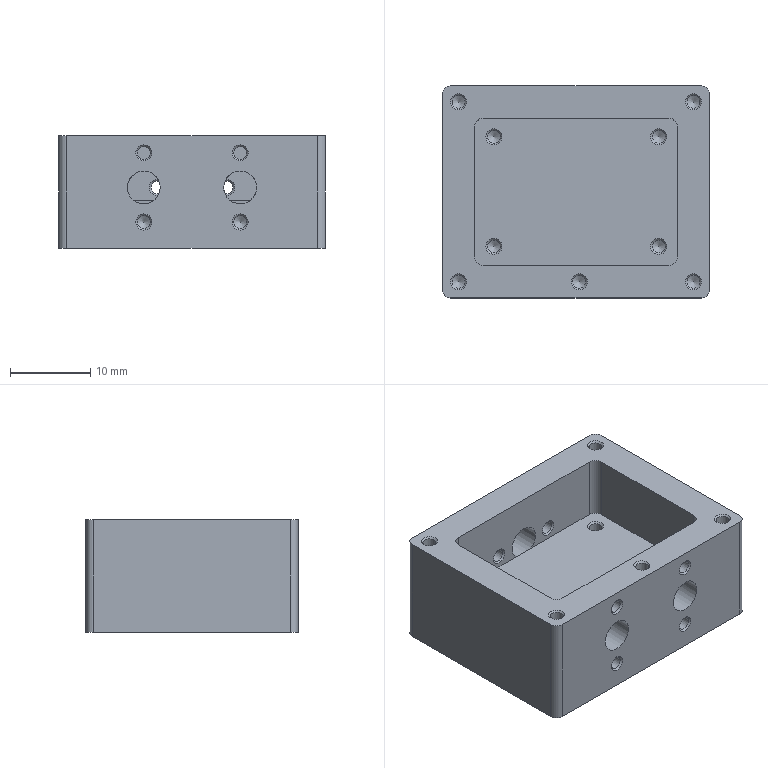Part | STEP file | 1 to 2 power divider cavity | 1 solid | 82 faces | box 33.2 x 26.38 x 14 mm | volume 8149 mm3 | cone 38 | cylinder 30 | plane 14 | commonest cylinder face diameters 1.6 x15 2 x4 2.05 x4 2.2 x4 4.1 x3